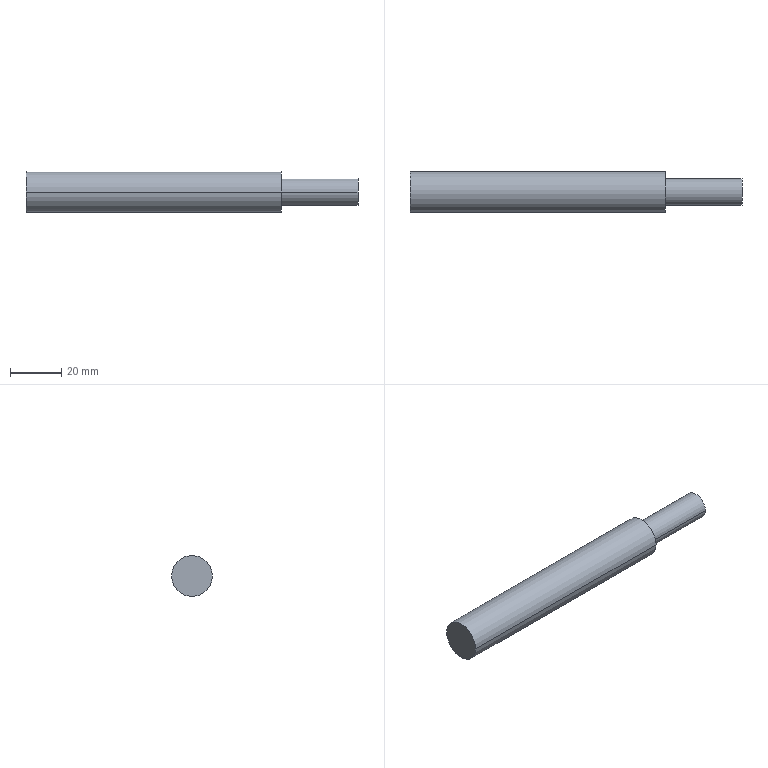Part | STEP file | screw_STEP.stp | 1 solid | 7 faces | box 130 x 16 x 16 mm | volume 22700 mm3 | cylinder 4 | plane 3 | commonest cylinder face diameters 10.492 x2 16 x2
STEP:
#1=CARTESIAN_POINT('',(20.,5.246,0.));
#2=VERTEX_POINT('',#1);
#3=CARTESIAN_POINT('',(20.,-5.246,0.));
#4=VERTEX_POINT('',#3);
#5=CARTESIAN_POINT('',(20.,0.,0.));
#6=DIRECTION('',(1.,0.,0.));
#7=DIRECTION('',(0.,1.,0.));
#8=AXIS2_PLACEMENT_3D('',#5,#6,#7);
#9=CIRCLE('',#8,5.246);
#10=EDGE_CURVE('',#2,#4,#9,.T.);
#11=ORIENTED_EDGE('',*,*,#10,.T.);
#12=CARTESIAN_POINT('',(50.,-5.246,0.));
#13=VERTEX_POINT('',#12);
#14=CARTESIAN_POINT('',(20.,-5.246,0.));
#15=DIRECTION('',(1.,0.,0.));
#16=VECTOR('',#15,1000.);
#17=LINE('',#14,#16);
#18=EDGE_CURVE('',#4,#13,#17,.T.);
#19=ORIENTED_EDGE('',*,*,#18,.T.);
#20=CARTESIAN_POINT('',(50.,5.246,0.));
#21=VERTEX_POINT('',#20);
#22=CARTESIAN_POINT('',(50.,0.,0.));
#23=DIRECTION('',(1.,0.,0.));
#24=DIRECTION('',(0.,1.,0.));
#25=AXIS2_PLACEMENT_3D('',#22,#23,#24);
#26=CIRCLE('',#25,5.246);
#27=EDGE_CURVE('',#21,#13,#26,.T.);
#28=ORIENTED_EDGE('',*,*,#27,.F.);
#29=CARTESIAN_POINT('',(20.,5.246,0.));
#30=DIRECTION('',(1.,0.,0.));
#31=VECTOR('',#30,1000.);
#32=LINE('',#29,#31);
#33=EDGE_CURVE('',#2,#21,#32,.T.);
#34=ORIENTED_EDGE('',*,*,#33,.F.);
#35=EDGE_LOOP('',(#11,#19,#28,#34));
#36=FACE_OUTER_BOUND('',#35,.T.);
#37=CARTESIAN_POINT('',(20.,0.,0.));
#38=DIRECTION('',(1.,0.,0.));
#39=DIRECTION('',(0.,1.,0.));
#40=AXIS2_PLACEMENT_3D('',#37,#38,#39);
#41=CYLINDRICAL_SURFACE('',#40,5.246);
#42=ADVANCED_FACE('',(#36),#41,.T.);
#43=CARTESIAN_POINT('',(20.,8.,0.));
#44=VERTEX_POINT('',#43);
#45=CARTESIAN_POINT('',(20.,-8.,0.));
#46=VERTEX_POINT('',#45);
#47=CARTESIAN_POINT('',(20.,0.,0.));
#48=DIRECTION('',(1.,0.,0.));
#49=DIRECTION('',(0.,1.,0.));
#50=AXIS2_PLACEMENT_3D('',#47,#48,#49);
#51=CIRCLE('',#50,8.);
#52=EDGE_CURVE('',#44,#46,#51,.T.);
#53=ORIENTED_EDGE('',*,*,#52,.F.);
#54=CARTESIAN_POINT('',(-80.,8.,0.));
#55=VERTEX_POINT('',#54);
#56=CARTESIAN_POINT('',(50.,8.,0.));
#57=DIRECTION('',(-1.,0.,0.));
#58=VECTOR('',#57,1000.);
#59=LINE('',#56,#58);
#60=EDGE_CURVE('',#44,#55,#59,.T.);
#61=ORIENTED_EDGE('',*,*,#60,.T.);
#62=CARTESIAN_POINT('',(-80.,-8.,0.));
#63=VERTEX_POINT('',#62);
#64=CARTESIAN_POINT('',(-80.,0.,0.));
#65=DIRECTION('',(-1.,0.,0.));
#66=DIRECTION('',(0.,-1.,0.));
#67=AXIS2_PLACEMENT_3D('',#64,#65,#66);
#68=CIRCLE('',#67,8.);
#69=EDGE_CURVE('',#63,#55,#68,.T.);
#70=ORIENTED_EDGE('',*,*,#69,.F.);
#71=CARTESIAN_POINT('',(50.,-8.,0.));
#72=DIRECTION('',(-1.,0.,0.));
#73=VECTOR('',#72,1000.);
#74=LINE('',#71,#73);
#75=EDGE_CURVE('',#46,#63,#74,.T.);
#76=ORIENTED_EDGE('',*,*,#75,.F.);
#77=EDGE_LOOP('',(#53,#61,#70,#76));
#78=FACE_OUTER_BOUND('',#77,.T.);
#79=CARTESIAN_POINT('',(50.,0.,0.));
#80=DIRECTION('',(-1.,0.,0.));
#81=DIRECTION('',(0.,-1.,0.));
#82=AXIS2_PLACEMENT_3D('',#79,#80,#81);
#83=CYLINDRICAL_SURFACE('',#82,8.);
#84=ADVANCED_FACE('',(#78),#83,.T.);
#85=ORIENTED_EDGE('',*,*,#60,.F.);
#86=CARTESIAN_POINT('',(20.,0.,0.));
#87=DIRECTION('',(1.,0.,0.));
#88=DIRECTION('',(0.,1.,0.));
#89=AXIS2_PLACEMENT_3D('',#86,#87,#88);
#90=CIRCLE('',#89,8.);
#91=EDGE_CURVE('',#46,#44,#90,.T.);
#92=ORIENTED_EDGE('',*,*,#91,.F.);
#93=ORIENTED_EDGE('',*,*,#75,.T.);
#94=CARTESIAN_POINT('',(-80.,0.,0.));
#95=DIRECTION('',(-1.,0.,0.));
#96=DIRECTION('',(0.,-1.,0.));
#97=AXIS2_PLACEMENT_3D('',#94,#95,#96);
#98=CIRCLE('',#97,8.);
#99=EDGE_CURVE('',#55,#63,#98,.T.);
#100=ORIENTED_EDGE('',*,*,#99,.F.);
#101=EDGE_LOOP('',(#85,#92,#93,#100));
#102=FACE_OUTER_BOUND('',#101,.T.);
#103=CARTESIAN_POINT('',(50.,0.,0.));
#104=DIRECTION('',(-1.,0.,0.));
#105=DIRECTION('',(0.,-1.,0.));
#106=AXIS2_PLACEMENT_3D('',#103,#104,#105);
#107=CYLINDRICAL_SURFACE('',#106,8.);
#108=ADVANCED_FACE('',(#102),#107,.T.);
#109=ORIENTED_EDGE('',*,*,#69,.T.);
#110=ORIENTED_EDGE('',*,*,#99,.T.);
#111=EDGE_LOOP('',(#109,#110));
#112=FACE_OUTER_BOUND('',#111,.T.);
#113=CARTESIAN_POINT('',(-80.,0.,0.));
#114=DIRECTION('',(-1.,0.,0.));
#115=DIRECTION('',(0.,-1.,0.));
#116=AXIS2_PLACEMENT_3D('',#113,#114,#115);
#117=PLANE('',#116);
#118=ADVANCED_FACE('',(#112),#117,.T.);
#119=ORIENTED_EDGE('',*,*,#10,.F.);
#120=CARTESIAN_POINT('',(20.,0.,0.));
#121=DIRECTION('',(1.,0.,0.));
#122=DIRECTION('',(0.,1.,0.));
#123=AXIS2_PLACEMENT_3D('',#120,#121,#122);
#124=CIRCLE('',#123,5.246);
#125=EDGE_CURVE('',#4,#2,#124,.T.);
#126=ORIENTED_EDGE('',*,*,#125,.F.);
#127=EDGE_LOOP('',(#119,#126));
#128=FACE_BOUND('',#127,.T.);
#129=ORIENTED_EDGE('',*,*,#91,.T.);
#130=ORIENTED_EDGE('',*,*,#52,.T.);
#131=EDGE_LOOP('',(#129,#130));
#132=FACE_OUTER_BOUND('',#131,.T.);
#133=CARTESIAN_POINT('',(20.,0.,0.));
#134=DIRECTION('',(1.,0.,0.));
#135=DIRECTION('',(0.,1.,0.));
#136=AXIS2_PLACEMENT_3D('',#133,#134,#135);
#137=PLANE('',#136);
#138=ADVANCED_FACE('',(#128,#132),#137,.T.);
#139=ORIENTED_EDGE('',*,*,#18,.F.);
#140=ORIENTED_EDGE('',*,*,#125,.T.);
#141=ORIENTED_EDGE('',*,*,#33,.T.);
#142=CARTESIAN_POINT('',(50.,0.,0.));
#143=DIRECTION('',(1.,0.,0.));
#144=DIRECTION('',(0.,1.,0.));
#145=AXIS2_PLACEMENT_3D('',#142,#143,#144);
#146=CIRCLE('',#145,5.246);
#147=EDGE_CURVE('',#13,#21,#146,.T.);
#148=ORIENTED_EDGE('',*,*,#147,.F.);
#149=EDGE_LOOP('',(#139,#140,#141,#148));
#150=FACE_OUTER_BOUND('',#149,.T.);
#151=CARTESIAN_POINT('',(20.,0.,0.));
#152=DIRECTION('',(1.,0.,0.));
#153=DIRECTION('',(0.,1.,0.));
#154=AXIS2_PLACEMENT_3D('',#151,#152,#153);
#155=CYLINDRICAL_SURFACE('',#154,5.246);
#156=ADVANCED_FACE('',(#150),#155,.T.);
#157=ORIENTED_EDGE('',*,*,#27,.T.);
#158=ORIENTED_EDGE('',*,*,#147,.T.);
#159=EDGE_LOOP('',(#157,#158));
#160=FACE_OUTER_BOUND('',#159,.T.);
#161=CARTESIAN_POINT('',(50.,0.,0.));
#162=DIRECTION('',(-1.,0.,0.));
#163=DIRECTION('',(0.,0.,1.));
#164=AXIS2_PLACEMENT_3D('',#161,#162,#163);
#165=PLANE('',#164);
#166=ADVANCED_FACE('',(#160),#165,.F.);
#167=CLOSED_SHELL('',(#42,#84,#108,#118,#138,#156,#166));
#168=MANIFOLD_SOLID_BREP('',#167);
#169=CARTESIAN_POINT('',(0.,0.,0.));
#170=DIRECTION('',(0.,0.,1.));
#171=DIRECTION('',(1.,0.,0.));
#172=AXIS2_PLACEMENT_3D('',#169,#170,#171);
#173=(LENGTH_UNIT()NAMED_UNIT(*)SI_UNIT(.MILLI.,.METRE.));
#174=UNCERTAINTY_MEASURE_WITH_UNIT(LENGTH_MEASURE(0.00001),#173,'','');
#175=(NAMED_UNIT(*)PLANE_ANGLE_UNIT()SI_UNIT($,.RADIAN.));
#176=(NAMED_UNIT(*)SI_UNIT($,.STERADIAN.)SOLID_ANGLE_UNIT());
#177=(GEOMETRIC_REPRESENTATION_CONTEXT(3)GLOBAL_UNCERTAINTY_ASSIGNED_CONTEXT((#174))GLOBAL_UNIT_ASSIGNED_CONTEXT((#173,#175,#176))REPRESENTATION_CONTEXT('',''));
#178=ADVANCED_BREP_SHAPE_REPRESENTATION('',(#168,#172),#177);